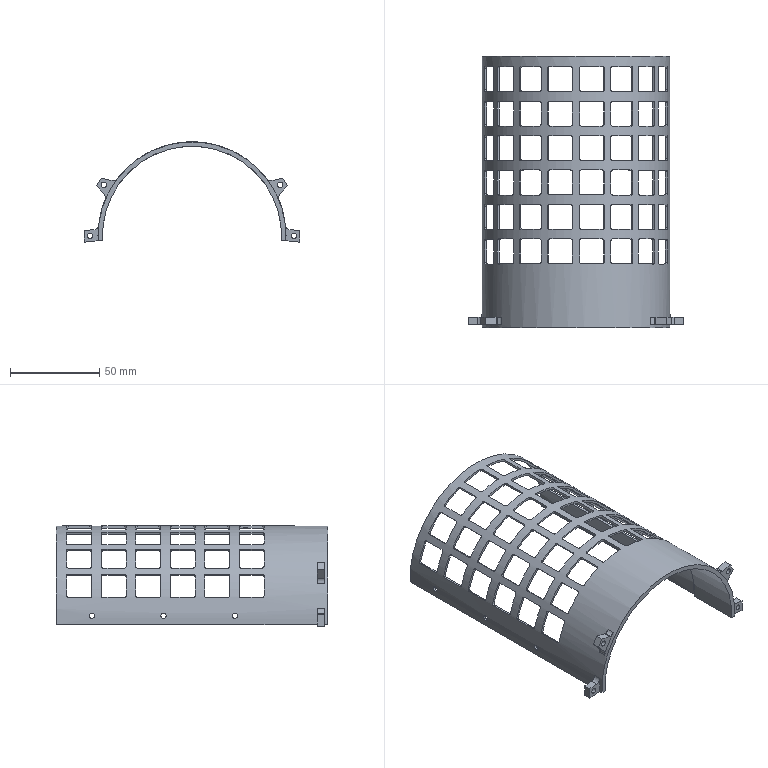Part | SolidWorks | features ICE 3, Fillet 2, Emboss 1, Extrusion 1 | 1 solid | 443 faces | box 120.4 x 151.9 x 56.149 mm | volume 26782 mm3 | plane 216 | spline 192 | cylinder 31 | torus 4 | commonest cylinder face diameters 3 x12 3.1 x8 6 x8 100.2 x1 102.8 x1 105.2 x1